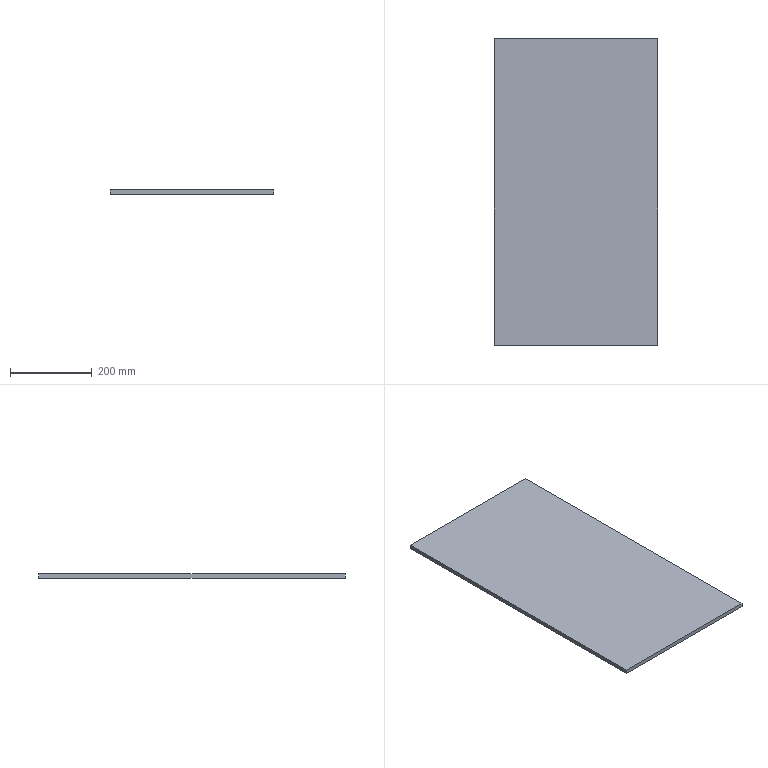Part | SolidWorks | features Extrusion 1 | 1 solid | 6 faces | box 400 x 749 x 10 mm | volume 2996000 mm3 | plane 6
STEP:
#1=CARTESIAN_POINT('',(-200.,374.5,-5.));
#2=VERTEX_POINT('',#1);
#3=CARTESIAN_POINT('',(-200.,-374.5,-5.));
#4=VERTEX_POINT('',#3);
#5=CARTESIAN_POINT('',(-200.,374.5,-5.));
#6=DIRECTION('',(0.,-1.,0.));
#7=VECTOR('',#6,1000.);
#8=LINE('',#5,#7);
#9=EDGE_CURVE('',#2,#4,#8,.T.);
#10=ORIENTED_EDGE('',*,*,#9,.T.);
#11=CARTESIAN_POINT('',(-200.,-374.5,5.));
#12=VERTEX_POINT('',#11);
#13=CARTESIAN_POINT('',(-200.,-374.5,5.));
#14=DIRECTION('',(0.,0.,-1.));
#15=VECTOR('',#14,1000.);
#16=LINE('',#13,#15);
#17=EDGE_CURVE('',#12,#4,#16,.T.);
#18=ORIENTED_EDGE('',*,*,#17,.F.);
#19=CARTESIAN_POINT('',(-200.,374.5,5.));
#20=VERTEX_POINT('',#19);
#21=CARTESIAN_POINT('',(-200.,374.5,5.));
#22=DIRECTION('',(0.,-1.,0.));
#23=VECTOR('',#22,1000.);
#24=LINE('',#21,#23);
#25=EDGE_CURVE('',#20,#12,#24,.T.);
#26=ORIENTED_EDGE('',*,*,#25,.F.);
#27=CARTESIAN_POINT('',(-200.,374.5,5.));
#28=DIRECTION('',(0.,0.,-1.));
#29=VECTOR('',#28,1000.);
#30=LINE('',#27,#29);
#31=EDGE_CURVE('',#20,#2,#30,.T.);
#32=ORIENTED_EDGE('',*,*,#31,.T.);
#33=EDGE_LOOP('',(#10,#18,#26,#32));
#34=FACE_OUTER_BOUND('',#33,.T.);
#35=CARTESIAN_POINT('',(-200.,374.5,5.));
#36=DIRECTION('',(1.,0.,0.));
#37=DIRECTION('',(0.,1.,0.));
#38=AXIS2_PLACEMENT_3D('',#35,#36,#37);
#39=PLANE('',#38);
#40=ADVANCED_FACE('',(#34),#39,.F.);
#41=CARTESIAN_POINT('',(200.,-374.5,-5.));
#42=VERTEX_POINT('',#41);
#43=CARTESIAN_POINT('',(-200.,-374.5,-5.));
#44=DIRECTION('',(1.,0.,0.));
#45=VECTOR('',#44,1000.);
#46=LINE('',#43,#45);
#47=EDGE_CURVE('',#4,#42,#46,.T.);
#48=ORIENTED_EDGE('',*,*,#47,.T.);
#49=CARTESIAN_POINT('',(200.,-374.5,5.));
#50=VERTEX_POINT('',#49);
#51=CARTESIAN_POINT('',(200.,-374.5,5.));
#52=DIRECTION('',(0.,0.,-1.));
#53=VECTOR('',#52,1000.);
#54=LINE('',#51,#53);
#55=EDGE_CURVE('',#50,#42,#54,.T.);
#56=ORIENTED_EDGE('',*,*,#55,.F.);
#57=CARTESIAN_POINT('',(-200.,-374.5,5.));
#58=DIRECTION('',(1.,0.,0.));
#59=VECTOR('',#58,1000.);
#60=LINE('',#57,#59);
#61=EDGE_CURVE('',#12,#50,#60,.T.);
#62=ORIENTED_EDGE('',*,*,#61,.F.);
#63=ORIENTED_EDGE('',*,*,#17,.T.);
#64=EDGE_LOOP('',(#48,#56,#62,#63));
#65=FACE_OUTER_BOUND('',#64,.T.);
#66=CARTESIAN_POINT('',(-200.,-374.5,5.));
#67=DIRECTION('',(0.,1.,0.));
#68=DIRECTION('',(-1.,0.,0.));
#69=AXIS2_PLACEMENT_3D('',#66,#67,#68);
#70=PLANE('',#69);
#71=ADVANCED_FACE('',(#65),#70,.F.);
#72=CARTESIAN_POINT('',(200.,374.5,-5.));
#73=VERTEX_POINT('',#72);
#74=CARTESIAN_POINT('',(200.,374.5,-5.));
#75=DIRECTION('',(0.,1.,0.));
#76=VECTOR('',#75,1000.);
#77=LINE('',#74,#76);
#78=EDGE_CURVE('',#42,#73,#77,.T.);
#79=ORIENTED_EDGE('',*,*,#78,.T.);
#80=CARTESIAN_POINT('',(200.,374.5,5.));
#81=VERTEX_POINT('',#80);
#82=CARTESIAN_POINT('',(200.,374.5,5.));
#83=DIRECTION('',(0.,0.,-1.));
#84=VECTOR('',#83,1000.);
#85=LINE('',#82,#84);
#86=EDGE_CURVE('',#81,#73,#85,.T.);
#87=ORIENTED_EDGE('',*,*,#86,.F.);
#88=CARTESIAN_POINT('',(200.,374.5,5.));
#89=DIRECTION('',(0.,1.,0.));
#90=VECTOR('',#89,1000.);
#91=LINE('',#88,#90);
#92=EDGE_CURVE('',#50,#81,#91,.T.);
#93=ORIENTED_EDGE('',*,*,#92,.F.);
#94=ORIENTED_EDGE('',*,*,#55,.T.);
#95=EDGE_LOOP('',(#79,#87,#93,#94));
#96=FACE_OUTER_BOUND('',#95,.T.);
#97=CARTESIAN_POINT('',(200.,374.5,5.));
#98=DIRECTION('',(-1.,0.,0.));
#99=DIRECTION('',(0.,-1.,0.));
#100=AXIS2_PLACEMENT_3D('',#97,#98,#99);
#101=PLANE('',#100);
#102=ADVANCED_FACE('',(#96),#101,.F.);
#103=CARTESIAN_POINT('',(-200.,374.5,-5.));
#104=DIRECTION('',(-1.,0.,0.));
#105=VECTOR('',#104,1000.);
#106=LINE('',#103,#105);
#107=EDGE_CURVE('',#73,#2,#106,.T.);
#108=ORIENTED_EDGE('',*,*,#107,.T.);
#109=ORIENTED_EDGE('',*,*,#31,.F.);
#110=CARTESIAN_POINT('',(-200.,374.5,5.));
#111=DIRECTION('',(-1.,0.,0.));
#112=VECTOR('',#111,1000.);
#113=LINE('',#110,#112);
#114=EDGE_CURVE('',#81,#20,#113,.T.);
#115=ORIENTED_EDGE('',*,*,#114,.F.);
#116=ORIENTED_EDGE('',*,*,#86,.T.);
#117=EDGE_LOOP('',(#108,#109,#115,#116));
#118=FACE_OUTER_BOUND('',#117,.T.);
#119=CARTESIAN_POINT('',(-200.,374.5,5.));
#120=DIRECTION('',(0.,-1.,0.));
#121=DIRECTION('',(1.,0.,0.));
#122=AXIS2_PLACEMENT_3D('',#119,#120,#121);
#123=PLANE('',#122);
#124=ADVANCED_FACE('',(#118),#123,.F.);
#125=ORIENTED_EDGE('',*,*,#25,.T.);
#126=ORIENTED_EDGE('',*,*,#61,.T.);
#127=ORIENTED_EDGE('',*,*,#92,.T.);
#128=ORIENTED_EDGE('',*,*,#114,.T.);
#129=EDGE_LOOP('',(#125,#126,#127,#128));
#130=FACE_OUTER_BOUND('',#129,.T.);
#131=CARTESIAN_POINT('',(-200.,-374.5,5.));
#132=DIRECTION('',(0.,0.,1.));
#133=DIRECTION('',(1.,0.,0.));
#134=AXIS2_PLACEMENT_3D('',#131,#132,#133);
#135=PLANE('',#134);
#136=ADVANCED_FACE('',(#130),#135,.T.);
#137=ORIENTED_EDGE('',*,*,#9,.F.);
#138=ORIENTED_EDGE('',*,*,#107,.F.);
#139=ORIENTED_EDGE('',*,*,#78,.F.);
#140=ORIENTED_EDGE('',*,*,#47,.F.);
#141=EDGE_LOOP('',(#137,#138,#139,#140));
#142=FACE_OUTER_BOUND('',#141,.T.);
#143=CARTESIAN_POINT('',(-200.,-374.5,-5.));
#144=DIRECTION('',(0.,0.,1.));
#145=DIRECTION('',(1.,0.,0.));
#146=AXIS2_PLACEMENT_3D('',#143,#144,#145);
#147=PLANE('',#146);
#148=ADVANCED_FACE('',(#142),#147,.F.);
#149=CLOSED_SHELL('',(#40,#71,#102,#124,#136,#148));
#150=MANIFOLD_SOLID_BREP('',#149);
#151=CARTESIAN_POINT('',(0.,0.,0.));
#152=DIRECTION('',(0.,0.,1.));
#153=DIRECTION('',(1.,0.,0.));
#154=AXIS2_PLACEMENT_3D('',#151,#152,#153);
#155=(LENGTH_UNIT()NAMED_UNIT(*)SI_UNIT(.MILLI.,.METRE.));
#156=UNCERTAINTY_MEASURE_WITH_UNIT(LENGTH_MEASURE(0.00001),#155,'','');
#157=(NAMED_UNIT(*)PLANE_ANGLE_UNIT()SI_UNIT($,.RADIAN.));
#158=(NAMED_UNIT(*)SI_UNIT($,.STERADIAN.)SOLID_ANGLE_UNIT());
#159=(GEOMETRIC_REPRESENTATION_CONTEXT(3)GLOBAL_UNCERTAINTY_ASSIGNED_CONTEXT((#156))GLOBAL_UNIT_ASSIGNED_CONTEXT((#155,#157,#158))REPRESENTATION_CONTEXT('',''));
#160=ADVANCED_BREP_SHAPE_REPRESENTATION('',(#150,#154),#159);